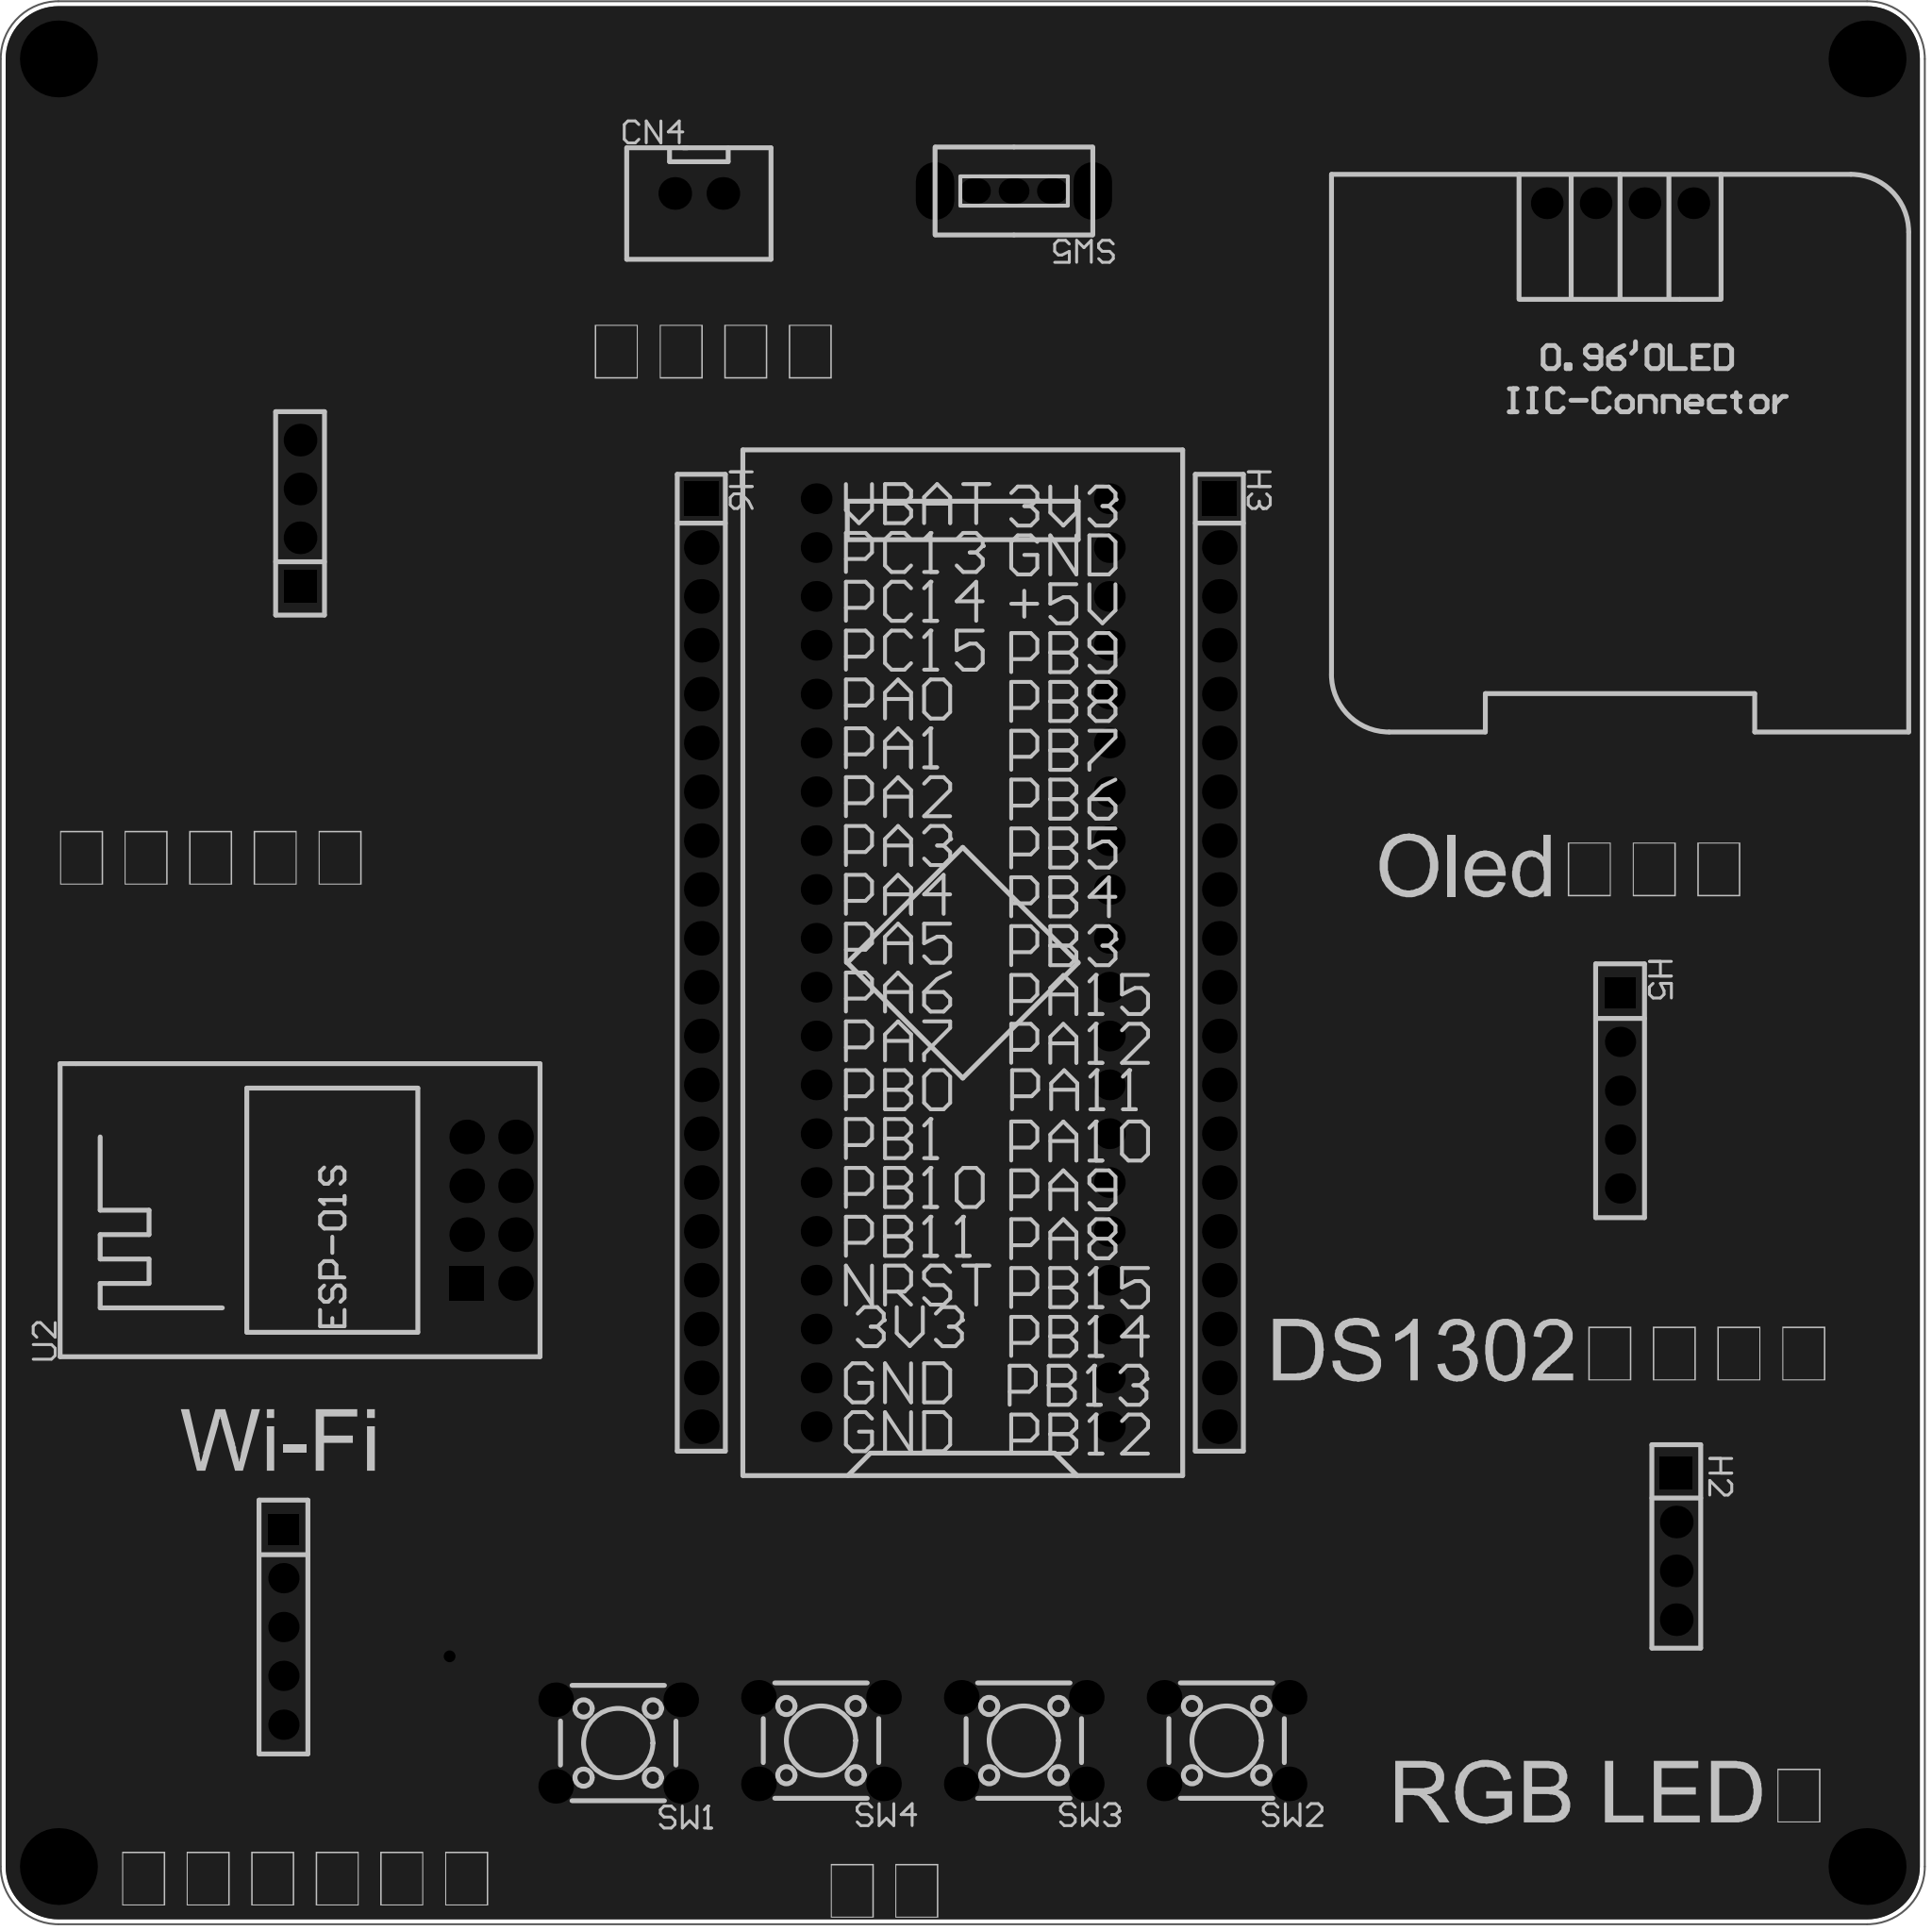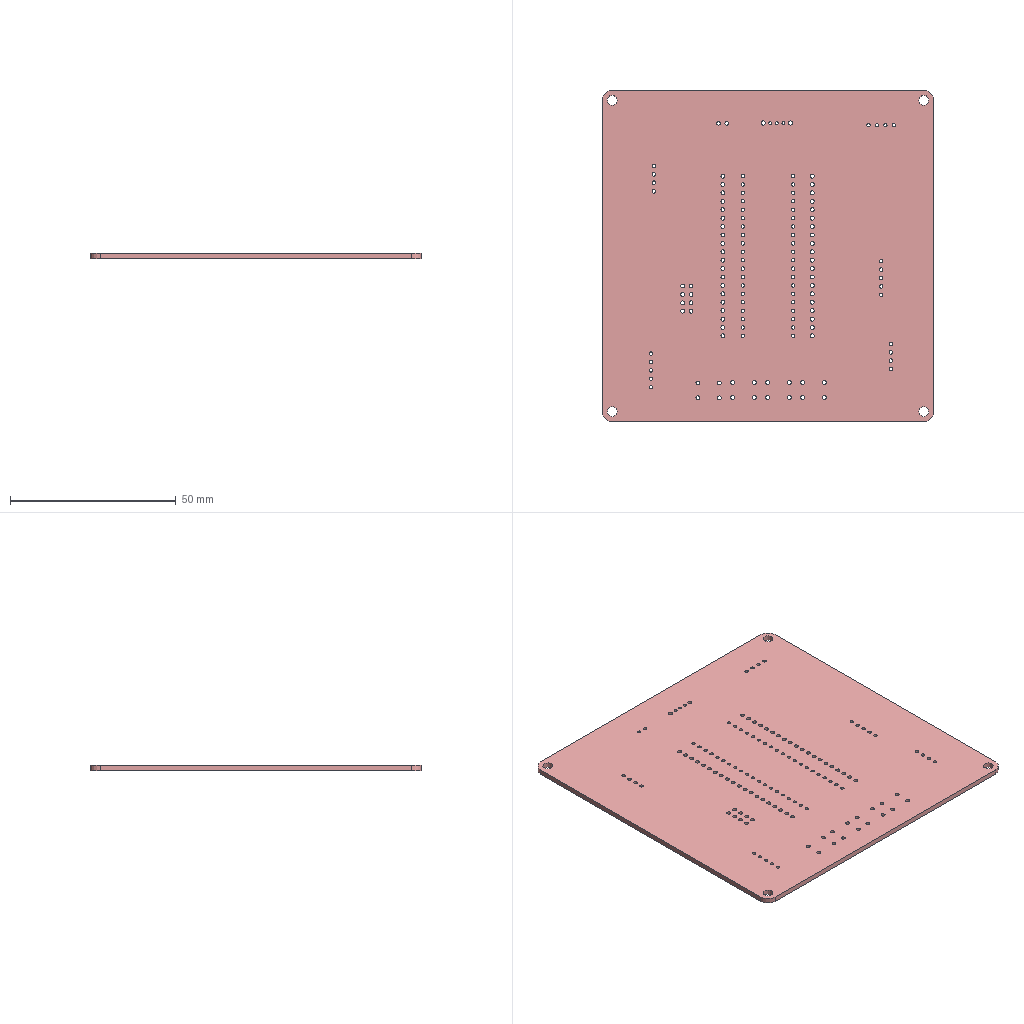Circuit board layout | Altium Designer | box 100 x 100 x 1.6 mm
Layer stack:
# Altium Designer layer stack of  (unit mm; dielectric type: 0 none, 1 core, 2 prepreg, 3 surface material)
index,name,kind,layer,copper_thickness_mm,dielectric_type,dielectric_thickness_mm,dielectric_material,dielectric_constant
0,Top Paste Mask Layer,other,,,,,,
1,Top Silkscreen Layer,other,,,,,,
2,Top Solder Mask Layer,dielectric,,,3,0.01,,3.3
3,Top Layer,copper,Top Layer,0.035,,,,
4,Dielectric1,dielectric,,,3,1.51,FR4,4.5
5,Bottom Layer,copper,Bottom Layer,0.035,,,,
6,Bottom Solder Mask Layer,dielectric,,,3,0.01,,3.3
7,Bottom Silkscreen Layer,other,,,,,,
8,Bottom Paste Mask Layer,other,,,,,,
# drill layer pairs: low layer,high layer
drill_pair,Top Layer,Bottom Layer
Part placement:
Designator,Comment,Layer,Footprint,Center-X(mm),Center-Y(mm),Rotation
U1,STM32F103C8T6-Card,TopLayer,CONN-TH_L53.3-W22.9_STM32F103C8T6-CARD,141.351,130.937,90
OLED1,,TopLayer,0.96OLED_4P,175.514,170.434,0
SW1,,TopLayer,SW-TH_4P-L6.0-W6.0-P4.50-LS6.5,123.444,90.36,180
SW2,,TopLayer,SW-TH_4P-L6.0-W6.0-P4.50-LS6.5,155.063,90.487,180
SW3,,TopLayer,SW-TH_4P-L6.0-W6.0-P4.50-LS6.5,144.524,90.487,180
SW4,,TopLayer,SW-TH_4P-L6.0-W6.0-P4.50-LS6.5,133.984,90.487,180
H4,,TopLayer,HDR-TH_4P-P2.54-V-F,106.909,154.305,90
H5,,TopLayer,HDR-TH_5P-P2.54-V-F,175.514,124.28,270
U2,ESP-01S,TopLayer,WIFIM-TH_ESP-01S,116.84,118.069,90
CN4,XH2.54*2P_直插,TopLayer,CONN-TH_2P-P2.50-XH2.54-2P,127.635,170.942,0
SW5,,TopLayer,拨动开关,144.01,171.069,180
H1,,TopLayer,HDR-TH_5P-P2.54-V-F,106.045,96.393,270
H2,,TopLayer,HDR-TH_4P-P2.54-V-F,178.435,100.584,270
H3,,TopLayer,HDR-TH_20P-P2.54-V-M-1,154.686,130.937,270
H6,,TopLayer,HDR-TH_20P-P2.54-V-M-1,127.762,130.937,270
Pad and via stacks:
# Altium Designer via and pad stacks of  (unit mm). Each distinct definition once, with the count of objects using it.
# via: kind,start_layer,end_layer,hole_mm,diameter_mm,mode(0 simple;1 top-mid-bottom;2 full stack),diameter_per_layer,count,example_net
# pad: kind,layer,hole_mm,hole_type(0 round;1 square;2 slot),plating,top_size,top_shape(1 round;2 rect;3 octagon;9 rounded rect),mid_size,bottom_size,mode,footprint,size_per_layer,count,example
pad,Multi-Layer,3,0,plated,4x4,1,4x4,4x4,0,,,4,1
pad,Multi-Layer,1,0,plated,1.6x1.6,1,1.6x1.6,1.6x1.6,0,CONN-TH_L53.3-W22.9_STM32F103C8T6-CARD,,40,U1.1
pad,Multi-Layer,1,0,plated,1.65x1.65,1,1.65x1.65,1.65x1.65,0,0.96OLED_4P,,4,OLED1.4
pad,Multi-Layer,1.2,0,plated,1.8x1.8,1,1.8x1.8,1.8x1.8,0,SW-TH_4P-L6.0-W6.0-P4.50-LS6.5,,16,SW1.1
pad,Multi-Layer,1.1,0,plated,1.7x1.7,2,1.7x1.7,1.7x1.7,0,HDR-TH_4P-P2.54-V-F,,2,H4.1
pad,Multi-Layer,1.1,0,plated,1.7x1.7,1,1.7x1.7,1.7x1.7,0,HDR-TH_4P-P2.54-V-F,,6,H4.2
pad,Multi-Layer,1.02,0,plated,1.575x1.575,1,1.575x1.575,1.575x1.575,0,HDR-TH_5P-P2.54-V-F,,8,H5.5
pad,Multi-Layer,1.02,0,plated,1.575x1.575,2,1.575x1.575,1.575x1.575,0,HDR-TH_5P-P2.54-V-F,,2,H5.1
pad,Multi-Layer,1.2,0,plated,1.8x1.8,2,1.8x1.8,1.8x1.8,0,WIFIM-TH_ESP-01S,,1,U2.1
pad,Multi-Layer,1.2,0,plated,1.8x1.8,1,1.8x1.8,1.8x1.8,0,WIFIM-TH_ESP-01S,,7,U2.2
pad,Multi-Layer,1.05,0,plated,1.7x1.7,1,1.7x1.7,1.7x1.7,0,CONN-TH_2P-P2.50-XH2.54-2P,,2,CN4.2
pad,Multi-Layer,0.8992,0,plated,1.6x1.3,1,1.6x1.3,1.6x1.3,0,\u00B2\u00A6\u00B6\u00AF\u00BF\u00AA\u00B9\u00D8,,3,SW5.1
pad,Multi-Layer,1.3,0,plated,3x1.999,1,3x1.999,3x1.999,0,\u00B2\u00A6\u00B6\u00AF\u00BF\u00AA\u00B9\u00D8,,2,SW5.4
pad,Multi-Layer,1.2,0,plated,1.8x1.8,1,1.8x1.8,1.8x1.8,0,HDR-TH_20P-P2.54-V-M-1,,38,H3.20
pad,Multi-Layer,1.2,0,plated,1.8x1.8,2,1.8x1.8,1.8x1.8,0,HDR-TH_20P-P2.54-V-M-1,,2,H3.1
via,Top Layer,Bottom Layer,0.3048,0.61,0,,1,PB11
Copper pours:
name,layer,net,type(0 solid;1 hatched;2 none)
Bottom Layer-GND,Bottom Layer,GND,0
Top Layer-GND,Top Layer,GND,0
Design rules, without the lines most boards share:
# Altium Designer design rules of  (exported by Altium Designer, unit mm)
# columns: name | kind | enabled | priority | scope1 | scope2 | descriptor | typed fields (field=value)
Copper_copperRegion_copperThickness1oz | 0 | disabled | 4 | All | All | Clearance Constraint (Gap=5.984mil) (Disabled)(All),(All) | gap=0.152
Copper_copperRegion_copperThickness1oz_1 | 63 | disabled | 4 | All | All | Board Clearance Constraint (Gap=0mil) (Disabled)(All) |
Copper_copperRegion_Copper_copperRegion | 0 | disabled | 5 | All | All | Clearance Constraint (Gap=5.984mil) (Disabled)(All),(All) | gap=0.152
Copper_copperRegion_Copper_copperRegion_1 | 63 | disabled | 5 | All | All | Board Clearance Constraint (Gap=0mil) (Disabled)(All) |
copperThickness1oz | 0 | enabled | 6 | All | All | Clearance Constraint (Gap=5.984mil) (All),(All) | gap=0.152
copperThickness1oz_1 | 63 | enabled | 6 | All | All | Board Clearance Constraint (Gap=0mil) (All) |
copperRegion_copperThickness1oz | 20 | disabled | 1 | All | All | Polygon Connect Rule(Relief Connect )(Conductor Width=10mil) (Relief Angle=90 Angle) (Entries=4) (Air Gap Width=10mil) (Disabled)(All),(All) | connect_style(0=relief,1=direct,2=none)=0 relief_conductor_width=0.254 relief_entries=4
copperRegion_Copper_copperRegion | 20 | disabled | 2 | All | All | Polygon Connect Rule(Relief Connect )(Conductor Width=10mil) (Relief Angle=90 Angle) (Entries=4) (Air Gap Width=10mil) (Disabled)(All),(All) | connect_style(0=relief,1=direct,2=none)=0 relief_conductor_width=0.254 relief_entries=4
copperRegion | 20 | enabled | 3 | All | All | Polygon Connect Rule(Relief Connect )(Conductor Width=10mil) (Relief Angle=90 Angle) (Entries=4) (Air Gap Width=10mil) (All),(All) | connect_style(0=relief,1=direct,2=none)=0 relief_conductor_width=0.254 relief_entries=4